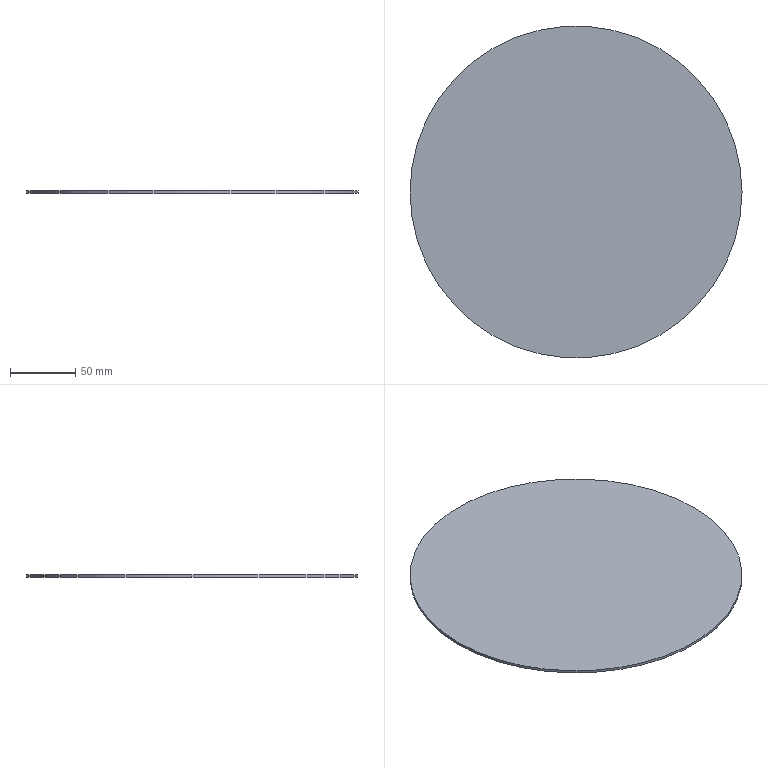Part | SolidWorks | features Extrusion 1 | 1 solid | 4 faces | box 254 x 254 x 2 mm | volume 101341 mm3 | cylinder 2 | plane 2 | commonest cylinder face diameters 254 x2
STEP:
#1=CARTESIAN_POINT('',(127.,0.,2.));
#2=VERTEX_POINT('',#1);
#3=CARTESIAN_POINT('',(-127.,0.,2.));
#4=VERTEX_POINT('',#3);
#5=CARTESIAN_POINT('',(0.,0.,2.));
#6=DIRECTION('',(0.,0.,1.));
#7=DIRECTION('',(1.,0.,0.));
#8=AXIS2_PLACEMENT_3D('',#5,#6,#7);
#9=CIRCLE('',#8,127.);
#10=EDGE_CURVE('',#2,#4,#9,.T.);
#11=ORIENTED_EDGE('',*,*,#10,.F.);
#12=CARTESIAN_POINT('',(127.,0.,0.));
#13=VERTEX_POINT('',#12);
#14=CARTESIAN_POINT('',(127.,0.,361.21));
#15=DIRECTION('',(0.,0.,-1.));
#16=VECTOR('',#15,1000.);
#17=LINE('',#14,#16);
#18=EDGE_CURVE('',#2,#13,#17,.T.);
#19=ORIENTED_EDGE('',*,*,#18,.T.);
#20=CARTESIAN_POINT('',(-127.,0.,0.));
#21=VERTEX_POINT('',#20);
#22=CARTESIAN_POINT('',(0.,0.,0.));
#23=DIRECTION('',(0.,0.,1.));
#24=DIRECTION('',(1.,0.,0.));
#25=AXIS2_PLACEMENT_3D('',#22,#23,#24);
#26=CIRCLE('',#25,127.);
#27=EDGE_CURVE('',#13,#21,#26,.T.);
#28=ORIENTED_EDGE('',*,*,#27,.T.);
#29=CARTESIAN_POINT('',(-127.,0.,361.21));
#30=DIRECTION('',(0.,0.,-1.));
#31=VECTOR('',#30,1000.);
#32=LINE('',#29,#31);
#33=EDGE_CURVE('',#4,#21,#32,.T.);
#34=ORIENTED_EDGE('',*,*,#33,.F.);
#35=EDGE_LOOP('',(#11,#19,#28,#34));
#36=FACE_OUTER_BOUND('',#35,.T.);
#37=CARTESIAN_POINT('',(0.,0.,361.21));
#38=DIRECTION('',(0.,0.,-1.));
#39=DIRECTION('',(-1.,0.,0.));
#40=AXIS2_PLACEMENT_3D('',#37,#38,#39);
#41=CYLINDRICAL_SURFACE('',#40,127.);
#42=ADVANCED_FACE('',(#36),#41,.T.);
#43=ORIENTED_EDGE('',*,*,#18,.F.);
#44=CARTESIAN_POINT('',(0.,0.,2.));
#45=DIRECTION('',(0.,0.,1.));
#46=DIRECTION('',(1.,0.,0.));
#47=AXIS2_PLACEMENT_3D('',#44,#45,#46);
#48=CIRCLE('',#47,127.);
#49=EDGE_CURVE('',#4,#2,#48,.T.);
#50=ORIENTED_EDGE('',*,*,#49,.F.);
#51=ORIENTED_EDGE('',*,*,#33,.T.);
#52=CARTESIAN_POINT('',(0.,0.,0.));
#53=DIRECTION('',(0.,0.,1.));
#54=DIRECTION('',(1.,0.,0.));
#55=AXIS2_PLACEMENT_3D('',#52,#53,#54);
#56=CIRCLE('',#55,127.);
#57=EDGE_CURVE('',#21,#13,#56,.T.);
#58=ORIENTED_EDGE('',*,*,#57,.T.);
#59=EDGE_LOOP('',(#43,#50,#51,#58));
#60=FACE_OUTER_BOUND('',#59,.T.);
#61=CARTESIAN_POINT('',(0.,0.,361.21));
#62=DIRECTION('',(0.,0.,-1.));
#63=DIRECTION('',(-1.,0.,0.));
#64=AXIS2_PLACEMENT_3D('',#61,#62,#63);
#65=CYLINDRICAL_SURFACE('',#64,127.);
#66=ADVANCED_FACE('',(#60),#65,.T.);
#67=ORIENTED_EDGE('',*,*,#57,.F.);
#68=ORIENTED_EDGE('',*,*,#27,.F.);
#69=EDGE_LOOP('',(#67,#68));
#70=FACE_OUTER_BOUND('',#69,.T.);
#71=CARTESIAN_POINT('',(0.,0.,0.));
#72=DIRECTION('',(0.,0.,1.));
#73=DIRECTION('',(1.,0.,0.));
#74=AXIS2_PLACEMENT_3D('',#71,#72,#73);
#75=PLANE('',#74);
#76=ADVANCED_FACE('',(#70),#75,.F.);
#77=ORIENTED_EDGE('',*,*,#49,.T.);
#78=ORIENTED_EDGE('',*,*,#10,.T.);
#79=EDGE_LOOP('',(#77,#78));
#80=FACE_OUTER_BOUND('',#79,.T.);
#81=CARTESIAN_POINT('',(-121.,0.,2.));
#82=DIRECTION('',(0.,0.,1.));
#83=DIRECTION('',(-1.,0.,0.));
#84=AXIS2_PLACEMENT_3D('',#81,#82,#83);
#85=PLANE('',#84);
#86=ADVANCED_FACE('',(#80),#85,.T.);
#87=CLOSED_SHELL('',(#42,#66,#76,#86));
#88=MANIFOLD_SOLID_BREP('',#87);
#89=CARTESIAN_POINT('',(0.,0.,0.));
#90=DIRECTION('',(0.,0.,1.));
#91=DIRECTION('',(1.,0.,0.));
#92=AXIS2_PLACEMENT_3D('',#89,#90,#91);
#93=(LENGTH_UNIT()NAMED_UNIT(*)SI_UNIT(.MILLI.,.METRE.));
#94=UNCERTAINTY_MEASURE_WITH_UNIT(LENGTH_MEASURE(0.00001),#93,'','');
#95=(NAMED_UNIT(*)PLANE_ANGLE_UNIT()SI_UNIT($,.RADIAN.));
#96=(NAMED_UNIT(*)SI_UNIT($,.STERADIAN.)SOLID_ANGLE_UNIT());
#97=(GEOMETRIC_REPRESENTATION_CONTEXT(3)GLOBAL_UNCERTAINTY_ASSIGNED_CONTEXT((#94))GLOBAL_UNIT_ASSIGNED_CONTEXT((#93,#95,#96))REPRESENTATION_CONTEXT('',''));
#98=ADVANCED_BREP_SHAPE_REPRESENTATION('',(#88,#92),#97);